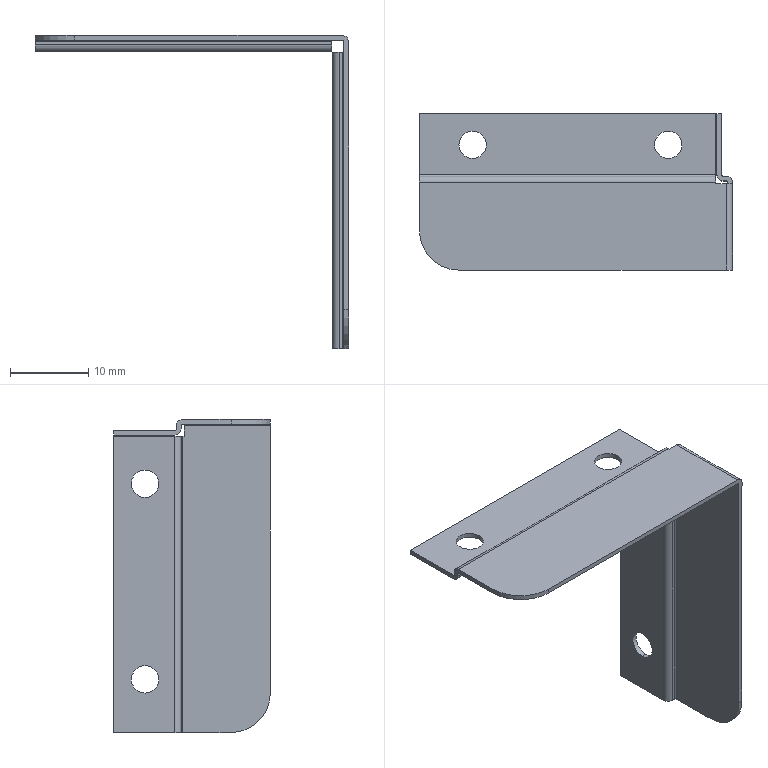Part | SolidWorks | features BaseBody 1 | 1 solid | 40 faces | box 40 x 20 x 40 mm | volume 945.968 mm3 | cylinder 20 | plane 20 | commonest cylinder face diameters 3.5 x8 0.4 x5 1.6 x5 10 x2
STEP:
#1=CARTESIAN_POINT('',(-9.96,6.,-2.));
#2=VERTEX_POINT('',#1);
#3=CARTESIAN_POINT('',(-6.46,6.,-2.));
#4=VERTEX_POINT('',#3);
#5=CARTESIAN_POINT('',(-8.21,6.,-2.));
#6=DIRECTION('',(0.,0.,1.));
#7=DIRECTION('',(1.,0.,0.));
#8=AXIS2_PLACEMENT_3D('',#5,#6,#7);
#9=CIRCLE('',#8,1.75);
#10=EDGE_CURVE('',#2,#4,#9,.T.);
#11=ORIENTED_EDGE('',*,*,#10,.F.);
#12=CARTESIAN_POINT('',(-9.96,6.,-1.4));
#13=VERTEX_POINT('',#12);
#14=CARTESIAN_POINT('',(-9.96,6.,-2.));
#15=DIRECTION('',(0.,0.,1.));
#16=VECTOR('',#15,1000.);
#17=LINE('',#14,#16);
#18=EDGE_CURVE('',#2,#13,#17,.T.);
#19=ORIENTED_EDGE('',*,*,#18,.T.);
#20=CARTESIAN_POINT('',(-6.46,6.,-1.4));
#21=VERTEX_POINT('',#20);
#22=CARTESIAN_POINT('',(-8.21,6.,-1.4));
#23=DIRECTION('',(0.,0.,-1.));
#24=DIRECTION('',(1.,0.,0.));
#25=AXIS2_PLACEMENT_3D('',#22,#23,#24);
#26=CIRCLE('',#25,1.75);
#27=EDGE_CURVE('',#21,#13,#26,.T.);
#28=ORIENTED_EDGE('',*,*,#27,.F.);
#29=CARTESIAN_POINT('',(-6.46,6.,-2.));
#30=DIRECTION('',(0.,0.,1.));
#31=VECTOR('',#30,1000.);
#32=LINE('',#29,#31);
#33=EDGE_CURVE('',#4,#21,#32,.T.);
#34=ORIENTED_EDGE('',*,*,#33,.F.);
#35=EDGE_LOOP('',(#11,#19,#28,#34));
#36=FACE_OUTER_BOUND('',#35,.T.);
#37=CARTESIAN_POINT('',(-8.21,6.,-2.));
#38=DIRECTION('',(0.,0.,1.));
#39=DIRECTION('',(1.,0.,0.));
#40=AXIS2_PLACEMENT_3D('',#37,#38,#39);
#41=CYLINDRICAL_SURFACE('',#40,1.75);
#42=ADVANCED_FACE('',(#36),#41,.F.);
#43=CARTESIAN_POINT('',(-34.96,6.,-2.));
#44=VERTEX_POINT('',#43);
#45=CARTESIAN_POINT('',(-31.46,6.,-2.));
#46=VERTEX_POINT('',#45);
#47=CARTESIAN_POINT('',(-33.21,6.,-2.));
#48=DIRECTION('',(0.,0.,1.));
#49=DIRECTION('',(1.,0.,0.));
#50=AXIS2_PLACEMENT_3D('',#47,#48,#49);
#51=CIRCLE('',#50,1.75);
#52=EDGE_CURVE('',#44,#46,#51,.T.);
#53=ORIENTED_EDGE('',*,*,#52,.F.);
#54=CARTESIAN_POINT('',(-34.96,6.,-1.4));
#55=VERTEX_POINT('',#54);
#56=CARTESIAN_POINT('',(-34.96,6.,-2.));
#57=DIRECTION('',(0.,0.,1.));
#58=VECTOR('',#57,1000.);
#59=LINE('',#56,#58);
#60=EDGE_CURVE('',#44,#55,#59,.T.);
#61=ORIENTED_EDGE('',*,*,#60,.T.);
#62=CARTESIAN_POINT('',(-31.46,6.,-1.4));
#63=VERTEX_POINT('',#62);
#64=CARTESIAN_POINT('',(-33.21,6.,-1.4));
#65=DIRECTION('',(0.,0.,-1.));
#66=DIRECTION('',(1.,0.,0.));
#67=AXIS2_PLACEMENT_3D('',#64,#65,#66);
#68=CIRCLE('',#67,1.75);
#69=EDGE_CURVE('',#63,#55,#68,.T.);
#70=ORIENTED_EDGE('',*,*,#69,.F.);
#71=CARTESIAN_POINT('',(-31.46,6.,-2.));
#72=DIRECTION('',(0.,0.,1.));
#73=VECTOR('',#72,1000.);
#74=LINE('',#71,#73);
#75=EDGE_CURVE('',#46,#63,#74,.T.);
#76=ORIENTED_EDGE('',*,*,#75,.F.);
#77=EDGE_LOOP('',(#53,#61,#70,#76));
#78=FACE_OUTER_BOUND('',#77,.T.);
#79=CARTESIAN_POINT('',(-33.21,6.,-2.));
#80=DIRECTION('',(0.,0.,1.));
#81=DIRECTION('',(1.,0.,0.));
#82=AXIS2_PLACEMENT_3D('',#79,#80,#81);
#83=CYLINDRICAL_SURFACE('',#82,1.75);
#84=ADVANCED_FACE('',(#78),#83,.F.);
#85=CARTESIAN_POINT('',(-2.,6.,-6.46));
#86=VERTEX_POINT('',#85);
#87=CARTESIAN_POINT('',(-2.,6.,-9.96));
#88=VERTEX_POINT('',#87);
#89=CARTESIAN_POINT('',(-2.,6.,-8.21));
#90=DIRECTION('',(1.,0.,0.));
#91=DIRECTION('',(0.,0.,-1.));
#92=AXIS2_PLACEMENT_3D('',#89,#90,#91);
#93=CIRCLE('',#92,1.75);
#94=EDGE_CURVE('',#86,#88,#93,.T.);
#95=ORIENTED_EDGE('',*,*,#94,.F.);
#96=CARTESIAN_POINT('',(-1.4,6.,-6.46));
#97=VERTEX_POINT('',#96);
#98=CARTESIAN_POINT('',(-2.,6.,-6.46));
#99=DIRECTION('',(1.,0.,0.));
#100=VECTOR('',#99,1000.);
#101=LINE('',#98,#100);
#102=EDGE_CURVE('',#86,#97,#101,.T.);
#103=ORIENTED_EDGE('',*,*,#102,.T.);
#104=CARTESIAN_POINT('',(-1.4,6.,-9.96));
#105=VERTEX_POINT('',#104);
#106=CARTESIAN_POINT('',(-1.4,6.,-8.21));
#107=DIRECTION('',(-1.,0.,0.));
#108=DIRECTION('',(0.,0.,-1.));
#109=AXIS2_PLACEMENT_3D('',#106,#107,#108);
#110=CIRCLE('',#109,1.75);
#111=EDGE_CURVE('',#105,#97,#110,.T.);
#112=ORIENTED_EDGE('',*,*,#111,.F.);
#113=CARTESIAN_POINT('',(-2.,6.,-9.96));
#114=DIRECTION('',(1.,0.,0.));
#115=VECTOR('',#114,1000.);
#116=LINE('',#113,#115);
#117=EDGE_CURVE('',#88,#105,#116,.T.);
#118=ORIENTED_EDGE('',*,*,#117,.F.);
#119=EDGE_LOOP('',(#95,#103,#112,#118));
#120=FACE_OUTER_BOUND('',#119,.T.);
#121=CARTESIAN_POINT('',(-2.,6.,-8.21));
#122=DIRECTION('',(1.,0.,0.));
#123=DIRECTION('',(0.,0.,-1.));
#124=AXIS2_PLACEMENT_3D('',#121,#122,#123);
#125=CYLINDRICAL_SURFACE('',#124,1.75);
#126=ADVANCED_FACE('',(#120),#125,.F.);
#127=CARTESIAN_POINT('',(-2.,6.,-31.46));
#128=VERTEX_POINT('',#127);
#129=CARTESIAN_POINT('',(-2.,6.,-34.96));
#130=VERTEX_POINT('',#129);
#131=CARTESIAN_POINT('',(-2.,6.,-33.21));
#132=DIRECTION('',(1.,0.,0.));
#133=DIRECTION('',(0.,0.,-1.));
#134=AXIS2_PLACEMENT_3D('',#131,#132,#133);
#135=CIRCLE('',#134,1.75);
#136=EDGE_CURVE('',#128,#130,#135,.T.);
#137=ORIENTED_EDGE('',*,*,#136,.F.);
#138=CARTESIAN_POINT('',(-1.4,6.,-31.46));
#139=VERTEX_POINT('',#138);
#140=CARTESIAN_POINT('',(-2.,6.,-31.46));
#141=DIRECTION('',(1.,0.,0.));
#142=VECTOR('',#141,1000.);
#143=LINE('',#140,#142);
#144=EDGE_CURVE('',#128,#139,#143,.T.);
#145=ORIENTED_EDGE('',*,*,#144,.T.);
#146=CARTESIAN_POINT('',(-1.4,6.,-34.96));
#147=VERTEX_POINT('',#146);
#148=CARTESIAN_POINT('',(-1.4,6.,-33.21));
#149=DIRECTION('',(-1.,0.,0.));
#150=DIRECTION('',(0.,0.,-1.));
#151=AXIS2_PLACEMENT_3D('',#148,#149,#150);
#152=CIRCLE('',#151,1.75);
#153=EDGE_CURVE('',#147,#139,#152,.T.);
#154=ORIENTED_EDGE('',*,*,#153,.F.);
#155=CARTESIAN_POINT('',(-2.,6.,-34.96));
#156=DIRECTION('',(1.,0.,0.));
#157=VECTOR('',#156,1000.);
#158=LINE('',#155,#157);
#159=EDGE_CURVE('',#130,#147,#158,.T.);
#160=ORIENTED_EDGE('',*,*,#159,.F.);
#161=EDGE_LOOP('',(#137,#145,#154,#160));
#162=FACE_OUTER_BOUND('',#161,.T.);
#163=CARTESIAN_POINT('',(-2.,6.,-33.21));
#164=DIRECTION('',(1.,0.,0.));
#165=DIRECTION('',(0.,0.,-1.));
#166=AXIS2_PLACEMENT_3D('',#163,#164,#165);
#167=CYLINDRICAL_SURFACE('',#166,1.75);
#168=ADVANCED_FACE('',(#162),#167,.F.);
#169=CARTESIAN_POINT('',(-0.8,-10.,0.));
#170=VERTEX_POINT('',#169);
#171=CARTESIAN_POINT('',(-0.8,1.,0.));
#172=VERTEX_POINT('',#171);
#173=CARTESIAN_POINT('',(-0.8,10.,0.));
#174=DIRECTION('',(0.,1.,0.));
#175=VECTOR('',#174,1000.);
#176=LINE('',#173,#175);
#177=EDGE_CURVE('',#170,#172,#176,.T.);
#178=ORIENTED_EDGE('',*,*,#177,.T.);
#179=CARTESIAN_POINT('',(-2.15,1.,0.));
#180=VERTEX_POINT('',#179);
#181=CARTESIAN_POINT('',(0.,1.,0.));
#182=DIRECTION('',(-1.,0.,0.));
#183=VECTOR('',#182,1000.);
#184=LINE('',#181,#183);
#185=EDGE_CURVE('',#172,#180,#184,.T.);
#186=ORIENTED_EDGE('',*,*,#185,.T.);
#187=CARTESIAN_POINT('',(-2.15,1.2,0.));
#188=VERTEX_POINT('',#187);
#189=CARTESIAN_POINT('',(-2.15,10.,0.));
#190=DIRECTION('',(0.,1.,0.));
#191=VECTOR('',#190,1000.);
#192=LINE('',#189,#191);
#193=EDGE_CURVE('',#180,#188,#192,.T.);
#194=ORIENTED_EDGE('',*,*,#193,.T.);
#195=CARTESIAN_POINT('',(-40.,1.2,0.));
#196=VERTEX_POINT('',#195);
#197=CARTESIAN_POINT('',(0.,1.2,0.));
#198=DIRECTION('',(-1.,0.,0.));
#199=VECTOR('',#198,1000.);
#200=LINE('',#197,#199);
#201=EDGE_CURVE('',#188,#196,#200,.T.);
#202=ORIENTED_EDGE('',*,*,#201,.T.);
#203=CARTESIAN_POINT('',(-40.,-5.,0.));
#204=VERTEX_POINT('',#203);
#205=CARTESIAN_POINT('',(-40.,10.,0.));
#206=DIRECTION('',(0.,-1.,0.));
#207=VECTOR('',#206,1000.);
#208=LINE('',#205,#207);
#209=EDGE_CURVE('',#196,#204,#208,.T.);
#210=ORIENTED_EDGE('',*,*,#209,.T.);
#211=CARTESIAN_POINT('',(-35.,-10.,0.));
#212=VERTEX_POINT('',#211);
#213=CARTESIAN_POINT('',(-35.,-5.,0.));
#214=DIRECTION('',(0.,0.,1.));
#215=DIRECTION('',(1.,0.,0.));
#216=AXIS2_PLACEMENT_3D('',#213,#214,#215);
#217=CIRCLE('',#216,5.);
#218=EDGE_CURVE('',#204,#212,#217,.T.);
#219=ORIENTED_EDGE('',*,*,#218,.T.);
#220=CARTESIAN_POINT('',(0.,-10.,0.));
#221=DIRECTION('',(1.,0.,0.));
#222=VECTOR('',#221,1000.);
#223=LINE('',#220,#222);
#224=EDGE_CURVE('',#212,#170,#223,.T.);
#225=ORIENTED_EDGE('',*,*,#224,.T.);
#226=EDGE_LOOP('',(#178,#186,#194,#202,#210,#219,#225));
#227=FACE_OUTER_BOUND('',#226,.T.);
#228=CARTESIAN_POINT('',(0.,10.,0.));
#229=DIRECTION('',(0.,0.,1.));
#230=DIRECTION('',(1.,0.,0.));
#231=AXIS2_PLACEMENT_3D('',#228,#229,#230);
#232=PLANE('',#231);
#233=ADVANCED_FACE('',(#227),#232,.T.);
#234=CARTESIAN_POINT('',(-0.8,1.,-0.6));
#235=VERTEX_POINT('',#234);
#236=CARTESIAN_POINT('',(-2.15,1.,-0.6));
#237=VERTEX_POINT('',#236);
#238=CARTESIAN_POINT('',(0.,1.,-0.6));
#239=DIRECTION('',(-1.,0.,0.));
#240=VECTOR('',#239,1000.);
#241=LINE('',#238,#240);
#242=EDGE_CURVE('',#235,#237,#241,.T.);
#243=ORIENTED_EDGE('',*,*,#242,.T.);
#244=CARTESIAN_POINT('',(-2.15,1.,0.));
#245=DIRECTION('',(0.,0.,1.));
#246=VECTOR('',#245,1000.);
#247=LINE('',#244,#246);
#248=EDGE_CURVE('',#237,#180,#247,.T.);
#249=ORIENTED_EDGE('',*,*,#248,.T.);
#250=ORIENTED_EDGE('',*,*,#185,.F.);
#251=CARTESIAN_POINT('',(0.,1.,-0.8));
#252=VERTEX_POINT('',#251);
#253=CARTESIAN_POINT('',(-0.8,1.,-0.8));
#254=DIRECTION('',(0.,-1.,0.));
#255=DIRECTION('',(0.,0.,-1.));
#256=AXIS2_PLACEMENT_3D('',#253,#254,#255);
#257=CIRCLE('',#256,0.8);
#258=EDGE_CURVE('',#252,#172,#257,.T.);
#259=ORIENTED_EDGE('',*,*,#258,.F.);
#260=CARTESIAN_POINT('',(0.,1.,-2.15));
#261=VERTEX_POINT('',#260);
#262=CARTESIAN_POINT('',(0.,1.,0.));
#263=DIRECTION('',(0.,0.,1.));
#264=VECTOR('',#263,1000.);
#265=LINE('',#262,#264);
#266=EDGE_CURVE('',#261,#252,#265,.T.);
#267=ORIENTED_EDGE('',*,*,#266,.F.);
#268=CARTESIAN_POINT('',(-0.6,1.,-2.15));
#269=VERTEX_POINT('',#268);
#270=CARTESIAN_POINT('',(0.,1.,-2.15));
#271=DIRECTION('',(-1.,0.,0.));
#272=VECTOR('',#271,1000.);
#273=LINE('',#270,#272);
#274=EDGE_CURVE('',#261,#269,#273,.T.);
#275=ORIENTED_EDGE('',*,*,#274,.T.);
#276=CARTESIAN_POINT('',(-0.6,1.,-0.8));
#277=VERTEX_POINT('',#276);
#278=CARTESIAN_POINT('',(-0.6,1.,0.));
#279=DIRECTION('',(0.,0.,1.));
#280=VECTOR('',#279,1000.);
#281=LINE('',#278,#280);
#282=EDGE_CURVE('',#269,#277,#281,.T.);
#283=ORIENTED_EDGE('',*,*,#282,.T.);
#284=CARTESIAN_POINT('',(-0.8,1.,-0.8));
#285=DIRECTION('',(0.,-1.,0.));
#286=DIRECTION('',(0.,0.,-1.));
#287=AXIS2_PLACEMENT_3D('',#284,#285,#286);
#288=CIRCLE('',#287,0.2);
#289=EDGE_CURVE('',#277,#235,#288,.T.);
#290=ORIENTED_EDGE('',*,*,#289,.T.);
#291=EDGE_LOOP('',(#243,#249,#250,#259,#267,#275,#283,#290));
#292=FACE_OUTER_BOUND('',#291,.T.);
#293=CARTESIAN_POINT('',(0.,1.,0.));
#294=DIRECTION('',(0.,1.,0.));
#295=DIRECTION('',(0.,0.,1.));
#296=AXIS2_PLACEMENT_3D('',#293,#294,#295);
#297=PLANE('',#296);
#298=ADVANCED_FACE('',(#292),#297,.T.);
#299=ORIENTED_EDGE('',*,*,#177,.F.);
#300=CARTESIAN_POINT('',(0.,-10.,-0.8));
#301=VERTEX_POINT('',#300);
#302=CARTESIAN_POINT('',(-0.8,-10.,-0.8));
#303=DIRECTION('',(0.,1.,0.));
#304=DIRECTION('',(0.,0.,-1.));
#305=AXIS2_PLACEMENT_3D('',#302,#303,#304);
#306=CIRCLE('',#305,0.8);
#307=EDGE_CURVE('',#170,#301,#306,.T.);
#308=ORIENTED_EDGE('',*,*,#307,.T.);
#309=CARTESIAN_POINT('',(0.,10.,-0.8));
#310=DIRECTION('',(0.,1.,0.));
#311=VECTOR('',#310,1000.);
#312=LINE('',#309,#311);
#313=EDGE_CURVE('',#301,#252,#312,.T.);
#314=ORIENTED_EDGE('',*,*,#313,.T.);
#315=ORIENTED_EDGE('',*,*,#258,.T.);
#316=EDGE_LOOP('',(#299,#308,#314,#315));
#317=FACE_OUTER_BOUND('',#316,.T.);
#318=CARTESIAN_POINT('',(-0.8,10.,-0.8));
#319=DIRECTION('',(0.,-1.,0.));
#320=DIRECTION('',(0.,0.,-1.));
#321=AXIS2_PLACEMENT_3D('',#318,#319,#320);
#322=CYLINDRICAL_SURFACE('',#321,0.8);
#323=ADVANCED_FACE('',(#317),#322,.T.);
#324=CARTESIAN_POINT('',(-35.,-10.,-0.6));
#325=VERTEX_POINT('',#324);
#326=CARTESIAN_POINT('',(-35.,-10.,-0.8));
#327=DIRECTION('',(0.,0.,1.));
#328=VECTOR('',#327,1000.);
#329=LINE('',#326,#328);
#330=EDGE_CURVE('',#325,#212,#329,.T.);
#331=ORIENTED_EDGE('',*,*,#330,.F.);
#332=CARTESIAN_POINT('',(-0.8,-10.,-0.6));
#333=VERTEX_POINT('',#332);
#334=CARTESIAN_POINT('',(-0.8,-10.,-0.6));
#335=DIRECTION('',(-1.,0.,0.));
#336=VECTOR('',#335,1000.);
#337=LINE('',#334,#336);
#338=EDGE_CURVE('',#333,#325,#337,.T.);
#339=ORIENTED_EDGE('',*,*,#338,.F.);
#340=CARTESIAN_POINT('',(-0.6,-10.,-0.8));
#341=VERTEX_POINT('',#340);
#342=CARTESIAN_POINT('',(-0.8,-10.,-0.8));
#343=DIRECTION('',(0.,1.,0.));
#344=DIRECTION('',(0.,0.,-1.));
#345=AXIS2_PLACEMENT_3D('',#342,#343,#344);
#346=CIRCLE('',#345,0.2);
#347=EDGE_CURVE('',#333,#341,#346,.T.);
#348=ORIENTED_EDGE('',*,*,#347,.T.);
#349=CARTESIAN_POINT('',(-0.6,-10.,-35.));
#350=VERTEX_POINT('',#349);
#351=CARTESIAN_POINT('',(-0.6,-10.,-0.6));
#352=DIRECTION('',(0.,0.,-1.));
#353=VECTOR('',#352,1000.);
#354=LINE('',#351,#353);
#355=EDGE_CURVE('',#341,#350,#354,.T.);
#356=ORIENTED_EDGE('',*,*,#355,.T.);
#357=CARTESIAN_POINT('',(0.,-10.,-35.));
#358=VERTEX_POINT('',#357);
#359=CARTESIAN_POINT('',(-0.8,-10.,-35.));
#360=DIRECTION('',(-1.,0.,0.));
#361=VECTOR('',#360,1000.);
#362=LINE('',#359,#361);
#363=EDGE_CURVE('',#358,#350,#362,.T.);
#364=ORIENTED_EDGE('',*,*,#363,.F.);
#365=CARTESIAN_POINT('',(0.,-10.,0.));
#366=DIRECTION('',(0.,0.,-1.));
#367=VECTOR('',#366,1000.);
#368=LINE('',#365,#367);
#369=EDGE_CURVE('',#301,#358,#368,.T.);
#370=ORIENTED_EDGE('',*,*,#369,.F.);
#371=ORIENTED_EDGE('',*,*,#307,.F.);
#372=ORIENTED_EDGE('',*,*,#224,.F.);
#373=EDGE_LOOP('',(#331,#339,#348,#356,#364,#370,#371,#372));
#374=FACE_OUTER_BOUND('',#373,.T.);
#375=CARTESIAN_POINT('',(-0.8,-10.,-0.8));
#376=DIRECTION('',(0.,1.,0.));
#377=DIRECTION('',(0.,0.,1.));
#378=AXIS2_PLACEMENT_3D('',#375,#376,#377);
#379=PLANE('',#378);
#380=ADVANCED_FACE('',(#374),#379,.F.);
#381=CARTESIAN_POINT('',(-40.,-5.,-0.6));
#382=VERTEX_POINT('',#381);
#383=CARTESIAN_POINT('',(-35.,-5.,-0.6));
#384=DIRECTION('',(0.,0.,1.));
#385=DIRECTION('',(1.,0.,0.));
#386=AXIS2_PLACEMENT_3D('',#383,#384,#385);
#387=CIRCLE('',#386,5.);
#388=EDGE_CURVE('',#382,#325,#387,.T.);
#389=ORIENTED_EDGE('',*,*,#388,.T.);
#390=ORIENTED_EDGE('',*,*,#330,.T.);
#391=ORIENTED_EDGE('',*,*,#218,.F.);
#392=CARTESIAN_POINT('',(-40.,-5.,-0.8));
#393=DIRECTION('',(0.,0.,-1.));
#394=VECTOR('',#393,1000.);
#395=LINE('',#392,#394);
#396=EDGE_CURVE('',#204,#382,#395,.T.);
#397=ORIENTED_EDGE('',*,*,#396,.T.);
#398=EDGE_LOOP('',(#389,#390,#391,#397));
#399=FACE_OUTER_BOUND('',#398,.T.);
#400=CARTESIAN_POINT('',(-35.,-5.,-0.8));
#401=DIRECTION('',(0.,0.,1.));
#402=DIRECTION('',(1.,0.,0.));
#403=AXIS2_PLACEMENT_3D('',#400,#401,#402);
#404=CYLINDRICAL_SURFACE('',#403,5.);
#405=ADVANCED_FACE('',(#399),#404,.T.);
#406=CARTESIAN_POINT('',(-40.,1.2,-0.6));
#407=VERTEX_POINT('',#406);
#408=CARTESIAN_POINT('',(-40.,10.,-0.6));
#409=DIRECTION('',(0.,-1.,0.));
#410=VECTOR('',#409,1000.);
#411=LINE('',#408,#410);
#412=EDGE_CURVE('',#407,#382,#411,.T.);
#413=ORIENTED_EDGE('',*,*,#412,.T.);
#414=ORIENTED_EDGE('',*,*,#396,.F.);
#415=ORIENTED_EDGE('',*,*,#209,.F.);
#416=CARTESIAN_POINT('',(-40.,2.,-0.8));
#417=VERTEX_POINT('',#416);
#418=CARTESIAN_POINT('',(-40.,1.2,-0.8));
#419=DIRECTION('',(1.,0.,0.));
#420=DIRECTION('',(0.,0.,1.));
#421=AXIS2_PLACEMENT_3D('',#418,#419,#420);
#422=CIRCLE('',#421,0.8);
#423=EDGE_CURVE('',#417,#196,#422,.T.);
#424=ORIENTED_EDGE('',*,*,#423,.F.);
#425=CARTESIAN_POINT('',(-40.,2.,-1.2));
#426=VERTEX_POINT('',#425);
#427=CARTESIAN_POINT('',(-40.,2.,-8.923));
#428=DIRECTION('',(0.,0.,1.));
#429=VECTOR('',#428,1000.);
#430=LINE('',#427,#429);
#431=EDGE_CURVE('',#426,#417,#430,.T.);
#432=ORIENTED_EDGE('',*,*,#431,.F.);
#433=CARTESIAN_POINT('',(-40.,2.2,-1.4));
#434=VERTEX_POINT('',#433);
#435=CARTESIAN_POINT('',(-40.,2.2,-1.2));
#436=DIRECTION('',(1.,0.,0.));
#437=DIRECTION('',(0.,0.,1.));
#438=AXIS2_PLACEMENT_3D('',#435,#436,#437);
#439=CIRCLE('',#438,0.2);
#440=EDGE_CURVE('',#426,#434,#439,.T.);
#441=ORIENTED_EDGE('',*,*,#440,.T.);
#442=CARTESIAN_POINT('',(-40.,10.,-1.4));
#443=VERTEX_POINT('',#442);
#444=CARTESIAN_POINT('',(-40.,9.246,-1.4));
#445=DIRECTION('',(0.,-1.,0.));
#446=VECTOR('',#445,1000.);
#447=LINE('',#444,#446);
#448=EDGE_CURVE('',#443,#434,#447,.T.);
#449=ORIENTED_EDGE('',*,*,#448,.F.);
#450=CARTESIAN_POINT('',(-40.,10.,-2.));
#451=VERTEX_POINT('',#450);
#452=CARTESIAN_POINT('',(-40.,10.,-1.4));
#453=DIRECTION('',(0.,0.,-1.));
#454=VECTOR('',#453,1000.);
#455=LINE('',#452,#454);
#456=EDGE_CURVE('',#443,#451,#455,.T.);
#457=ORIENTED_EDGE('',*,*,#456,.T.);
#458=CARTESIAN_POINT('',(-40.,2.2,-2.));
#459=VERTEX_POINT('',#458);
#460=CARTESIAN_POINT('',(-40.,9.246,-2.));
#461=DIRECTION('',(0.,-1.,0.));
#462=VECTOR('',#461,1000.);
#463=LINE('',#460,#462);
#464=EDGE_CURVE('',#451,#459,#463,.T.);
#465=ORIENTED_EDGE('',*,*,#464,.T.);
#466=CARTESIAN_POINT('',(-40.,1.4,-1.2));
#467=VERTEX_POINT('',#466);
#468=CARTESIAN_POINT('',(-40.,2.2,-1.2));
#469=DIRECTION('',(1.,0.,0.));
#470=DIRECTION('',(0.,0.,1.));
#471=AXIS2_PLACEMENT_3D('',#468,#469,#470);
#472=CIRCLE('',#471,0.8);
#473=EDGE_CURVE('',#467,#459,#472,.T.);
#474=ORIENTED_EDGE('',*,*,#473,.F.);
#475=CARTESIAN_POINT('',(-40.,1.4,-0.8));
#476=VERTEX_POINT('',#475);
#477=CARTESIAN_POINT('',(-40.,1.4,-8.923));
#478=DIRECTION('',(0.,0.,1.));
#479=VECTOR('',#478,1000.);
#480=LINE('',#477,#479);
#481=EDGE_CURVE('',#467,#476,#480,.T.);
#482=ORIENTED_EDGE('',*,*,#481,.T.);
#483=CARTESIAN_POINT('',(-40.,1.2,-0.8));
#484=DIRECTION('',(1.,0.,0.));
#485=DIRECTION('',(0.,0.,1.));
#486=AXIS2_PLACEMENT_3D('',#483,#484,#485);
#487=CIRCLE('',#486,0.2);
#488=EDGE_CURVE('',#476,#407,#487,.T.);
#489=ORIENTED_EDGE('',*,*,#488,.T.);
#490=EDGE_LOOP('',(#413,#414,#415,#424,#432,#441,#449,#457,#465,#474,#482,#489));
#491=FACE_OUTER_BOUND('',#490,.T.);
#492=CARTESIAN_POINT('',(-40.,10.,0.));
#493=DIRECTION('',(-1.,0.,0.));
#494=DIRECTION('',(0.,0.,1.));
#495=AXIS2_PLACEMENT_3D('',#492,#493,#494);
#496=PLANE('',#495);
#497=ADVANCED_FACE('',(#491),#496,.T.);
#498=CARTESIAN_POINT('',(-2.15,2.,-0.8));
#499=VERTEX_POINT('',#498);
#500=CARTESIAN_POINT('',(-2.15,1.2,-0.8));
#501=DIRECTION('',(-1.,0.,0.));
#502=DIRECTION('',(0.,0.,1.));
#503=AXIS2_PLACEMENT_3D('',#500,#501,#502);
#504=CIRCLE('',#503,0.8);
#505=EDGE_CURVE('',#188,#499,#504,.T.);
#506=ORIENTED_EDGE('',*,*,#505,.T.);
#507=CARTESIAN_POINT('',(16.786,2.,-0.8));
#508=DIRECTION('',(-1.,0.,0.));
#509=VECTOR('',#508,1000.);
#510=LINE('',#507,#509);
#511=EDGE_CURVE('',#499,#417,#510,.T.);
#512=ORIENTED_EDGE('',*,*,#511,.T.);
#513=ORIENTED_EDGE('',*,*,#423,.T.);
#514=ORIENTED_EDGE('',*,*,#201,.F.);
#515=EDGE_LOOP('',(#506,#512,#513,#514));
#516=FACE_OUTER_BOUND('',#515,.T.);
#517=CARTESIAN_POINT('',(16.786,1.2,-0.8));
#518=DIRECTION('',(-1.,0.,0.));
#519=DIRECTION('',(0.,0.,1.));
#520=AXIS2_PLACEMENT_3D('',#517,#518,#519);
#521=CYLINDRICAL_SURFACE('',#520,0.8);
#522=ADVANCED_FACE('',(#516),#521,.T.);
#523=ORIENTED_EDGE('',*,*,#193,.F.);
#524=ORIENTED_EDGE('',*,*,#248,.F.);
#525=CARTESIAN_POINT('',(-2.15,1.2,-0.6));
#526=VERTEX_POINT('',#525);
#527=CARTESIAN_POINT('',(-2.15,1.,-0.6));
#528=DIRECTION('',(0.,-1.,0.));
#529=VECTOR('',#528,1000.);
#530=LINE('',#527,#529);
#531=EDGE_CURVE('',#526,#237,#530,.T.);
#532=ORIENTED_EDGE('',*,*,#531,.F.);
#533=CARTESIAN_POINT('',(-2.15,1.4,-0.8));
#534=VERTEX_POINT('',#533);
#535=CARTESIAN_POINT('',(-2.15,1.2,-0.8));
#536=DIRECTION('',(-1.,0.,0.));
#537=DIRECTION('',(0.,0.,1.));
#538=AXIS2_PLACEMENT_3D('',#535,#536,#537);
#539=CIRCLE('',#538,0.2);
#540=EDGE_CURVE('',#526,#534,#539,.T.);
#541=ORIENTED_EDGE('',*,*,#540,.T.);
#542=CARTESIAN_POINT('',(-2.15,1.4,-1.2));
#543=VERTEX_POINT('',#542);
#544=CARTESIAN_POINT('',(-2.15,1.4,0.07701));
#545=DIRECTION('',(0.,0.,1.));
#546=VECTOR('',#545,1000.);
#547=LINE('',#544,#546);
#548=EDGE_CURVE('',#543,#534,#547,.T.);
#549=ORIENTED_EDGE('',*,*,#548,.F.);
#550=CARTESIAN_POINT('',(-2.15,2.2,-2.));
#551=VERTEX_POINT('',#550);
#552=CARTESIAN_POINT('',(-2.15,2.2,-1.2));
#553=DIRECTION('',(-1.,0.,0.));
#554=DIRECTION('',(0.,0.,1.));
#555=AXIS2_PLACEMENT_3D('',#552,#553,#554);
#556=CIRCLE('',#555,0.8);
#557=EDGE_CURVE('',#551,#543,#556,.T.);
#558=ORIENTED_EDGE('',*,*,#557,.F.);
#559=CARTESIAN_POINT('',(-2.15,10.,-2.));
#560=VERTEX_POINT('',#559);
#561=CARTESIAN_POINT('',(-2.15,0.246,-2.));
#562=DIRECTION('',(0.,-1.,0.));
#563=VECTOR('',#562,1000.);
#564=LINE('',#561,#563);
#565=EDGE_CURVE('',#560,#551,#564,.T.);
#566=ORIENTED_EDGE('',*,*,#565,.F.);
#567=CARTESIAN_POINT('',(-2.15,10.,-1.4));
#568=VERTEX_POINT('',#567);
#569=CARTESIAN_POINT('',(-2.15,10.,-2.2));
#570=DIRECTION('',(0.,0.,-1.));
#571=VECTOR('',#570,1000.);
#572=LINE('',#569,#571);
#573=EDGE_CURVE('',#568,#560,#572,.T.);
#574=ORIENTED_EDGE('',*,*,#573,.F.);
#575=CARTESIAN_POINT('',(-2.15,2.2,-1.4));
#576=VERTEX_POINT('',#575);
#577=CARTESIAN_POINT('',(-2.15,9.246,-1.4));
#578=DIRECTION('',(0.,1.,0.));
#579=VECTOR('',#578,1000.);
#580=LINE('',#577,#579);
#581=EDGE_CURVE('',#576,#568,#580,.T.);
#582=ORIENTED_EDGE('',*,*,#581,.F.);
#583=CARTESIAN_POINT('',(-2.15,2.,-1.2));
#584=VERTEX_POINT('',#583);
#585=CARTESIAN_POINT('',(-2.15,2.2,-1.2));
#586=DIRECTION('',(-1.,0.,0.));
#587=DIRECTION('',(0.,0.,1.));
#588=AXIS2_PLACEMENT_3D('',#585,#586,#587);
#589=CIRCLE('',#588,0.2);
#590=EDGE_CURVE('',#576,#584,#589,.T.);
#591=ORIENTED_EDGE('',*,*,#590,.T.);
#592=CARTESIAN_POINT('',(-2.15,2.,-8.923));
#593=DIRECTION('',(0.,0.,-1.));
#594=VECTOR('',#593,1000.);
#595=LINE('',#592,#594);
#596=EDGE_CURVE('',#499,#584,#595,.T.);
#597=ORIENTED_EDGE('',*,*,#596,.F.);
#598=ORIENTED_EDGE('',*,*,#505,.F.);
#599=EDGE_LOOP('',(#523,#524,#532,#541,#549,#558,#566,#574,#582,#591,#597,#598));
#600=FACE_OUTER_BOUND('',#599,.T.);
#601=CARTESIAN_POINT('',(-2.15,1.,-2.15));
#602=DIRECTION('',(-1.,0.,0.));
#603=DIRECTION('',(0.,0.,1.));
#604=AXIS2_PLACEMENT_3D('',#601,#602,#603);
#605=PLANE('',#604);
#606=ADVANCED_FACE('',(#600),#605,.F.);
#607=ORIENTED_EDGE('',*,*,#369,.T.);
#608=CARTESIAN_POINT('',(0.,-5.,-40.));
#609=VERTEX_POINT('',#608);
#610=CARTESIAN_POINT('',(0.,-5.,-35.));
#611=DIRECTION('',(1.,0.,0.));
#612=DIRECTION('',(0.,0.,-1.));
#613=AXIS2_PLACEMENT_3D('',#610,#611,#612);
#614=CIRCLE('',#613,5.);
#615=EDGE_CURVE('',#358,#609,#614,.T.);
#616=ORIENTED_EDGE('',*,*,#615,.T.);
#617=CARTESIAN_POINT('',(0.,1.2,-40.));
#618=VERTEX_POINT('',#617);
#619=CARTESIAN_POINT('',(0.,10.,-40.));
#620=DIRECTION('',(0.,1.,0.));
#621=VECTOR('',#620,1000.);
#622=LINE('',#619,#621);
#623=EDGE_CURVE('',#609,#618,#622,.T.);
#624=ORIENTED_EDGE('',*,*,#623,.T.);
#625=CARTESIAN_POINT('',(0.,1.2,-2.15));
#626=VERTEX_POINT('',#625);
#627=CARTESIAN_POINT('',(0.,1.2,0.));
#628=DIRECTION('',(0.,0.,1.));
#629=VECTOR('',#628,1000.);
#630=LINE('',#627,#629);
#631=EDGE_CURVE('',#618,#626,#630,.T.);
#632=ORIENTED_EDGE('',*,*,#631,.T.);
#633=CARTESIAN_POINT('',(0.,10.,-2.15));
#634=DIRECTION('',(0.,-1.,0.));
#635=VECTOR('',#634,1000.);
#636=LINE('',#633,#635);
#637=EDGE_CURVE('',#626,#261,#636,.T.);
#638=ORIENTED_EDGE('',*,*,#637,.T.);
#639=ORIENTED_EDGE('',*,*,#266,.T.);
#640=ORIENTED_EDGE('',*,*,#313,.F.);
#641=EDGE_LOOP('',(#607,#616,#624,#632,#638,#639,#640));
#642=FACE_OUTER_BOUND('',#641,.T.);
#643=CARTESIAN_POINT('',(0.,10.,0.));
#644=DIRECTION('',(1.,0.,0.));
#645=DIRECTION('',(0.,0.,-1.));
#646=AXIS2_PLACEMENT_3D('',#643,#644,#645);
#647=PLANE('',#646);
#648=ADVANCED_FACE('',(#642),#647,.T.);
#649=ORIENTED_EDGE('',*,*,#531,.T.);
#650=ORIENTED_EDGE('',*,*,#242,.F.);
#651=CARTESIAN_POINT('',(-0.8,10.,-0.6));
#652=DIRECTION('',(0.,1.,0.));
#653=VECTOR('',#652,1000.);
#654=LINE('',#651,#653);
#655=EDGE_CURVE('',#333,#235,#654,.T.);
#656=ORIENTED_EDGE('',*,*,#655,.F.);
#657=ORIENTED_EDGE('',*,*,#338,.T.);
#658=ORIENTED_EDGE('',*,*,#388,.F.);
#659=ORIENTED_EDGE('',*,*,#412,.F.);
#660=CARTESIAN_POINT('',(0.,1.2,-0.6));
#661=DIRECTION('',(-1.,0.,0.));
#662=VECTOR('',#661,1000.);
#663=LINE('',#660,#662);
#664=EDGE_CURVE('',#526,#407,#663,.T.);
#665=ORIENTED_EDGE('',*,*,#664,.F.);
#666=EDGE_LOOP('',(#649,#650,#656,#657,#658,#659,#665));
#667=FACE_OUTER_BOUND('',#666,.T.);
#668=CARTESIAN_POINT('',(0.,10.,-0.6));
#669=DIRECTION('',(0.,0.,1.));
#670=DIRECTION('',(1.,0.,0.));
#671=AXIS2_PLACEMENT_3D('',#668,#669,#670);
#672=PLANE('',#671);
#673=ADVANCED_FACE('',(#667),#672,.F.);
#674=ORIENTED_EDGE('',*,*,#431,.T.);
#675=ORIENTED_EDGE('',*,*,#511,.F.);
#676=ORIENTED_EDGE('',*,*,#596,.T.);
#677=CARTESIAN_POINT('',(0.,2.,-1.2));
#678=DIRECTION('',(-1.,0.,0.));
#679=VECTOR('',#678,1000.);
#680=LINE('',#677,#679);
#681=EDGE_CURVE('',#584,#426,#680,.T.);
#682=ORIENTED_EDGE('',*,*,#681,.T.);
#683=EDGE_LOOP('',(#674,#675,#676,#682));
#684=FACE_OUTER_BOUND('',#683,.T.);
#685=CARTESIAN_POINT('',(0.,2.,-8.923));
#686=DIRECTION('',(0.,1.,0.));
#687=DIRECTION('',(0.,0.,1.));
#688=AXIS2_PLACEMENT_3D('',#685,#686,#687);
#689=PLANE('',#688);
#690=ADVANCED_FACE('',(#684),#689,.T.);
#691=ORIENTED_EDGE('',*,*,#615,.F.);
#692=ORIENTED_EDGE('',*,*,#363,.T.);
#693=CARTESIAN_POINT('',(-0.6,-5.,-40.));
#694=VERTEX_POINT('',#693);
#695=CARTESIAN_POINT('',(-0.6,-5.,-35.));
#696=DIRECTION('',(1.,0.,0.));
#697=DIRECTION('',(0.,0.,-1.));
#698=AXIS2_PLACEMENT_3D('',#695,#696,#697);
#699=CIRCLE('',#698,5.);
#700=EDGE_CURVE('',#350,#694,#699,.T.);
#701=ORIENTED_EDGE('',*,*,#700,.T.);
#702=CARTESIAN_POINT('',(-0.8,-5.,-40.));
#703=DIRECTION('',(1.,0.,0.));
#704=VECTOR('',#703,1000.);
#705=LINE('',#702,#704);
#706=EDGE_CURVE('',#694,#609,#705,.T.);
#707=ORIENTED_EDGE('',*,*,#706,.T.);
#708=EDGE_LOOP('',(#691,#692,#701,#707));
#709=FACE_OUTER_BOUND('',#708,.T.);
#710=CARTESIAN_POINT('',(-0.8,-5.,-35.));
#711=DIRECTION('',(1.,0.,0.));
#712=DIRECTION('',(0.,0.,-1.));
#713=AXIS2_PLACEMENT_3D('',#710,#711,#712);
#714=CYLINDRICAL_SURFACE('',#713,5.);
#715=ADVANCED_FACE('',(#709),#714,.T.);
#716=CARTESIAN_POINT('',(-0.6,1.2,-2.15));
#717=VERTEX_POINT('',#716);
#718=CARTESIAN_POINT('',(-0.6,1.,-2.15));
#719=DIRECTION('',(0.,1.,0.));
#720=VECTOR('',#719,1000.);
#721=LINE('',#718,#720);
#722=EDGE_CURVE('',#269,#717,#721,.T.);
#723=ORIENTED_EDGE('',*,*,#722,.F.);
#724=ORIENTED_EDGE('',*,*,#274,.F.);
#725=ORIENTED_EDGE('',*,*,#637,.F.);
#726=CARTESIAN_POINT('',(-0.8,2.,-2.15));
#727=VERTEX_POINT('',#726);
#728=CARTESIAN_POINT('',(-0.8,1.2,-2.15));
#729=DIRECTION('',(0.,0.,-1.));
#730=DIRECTION('',(1.,0.,0.));
#731=AXIS2_PLACEMENT_3D('',#728,#729,#730);
#732=CIRCLE('',#731,0.8);
#733=EDGE_CURVE('',#727,#626,#732,.T.);
#734=ORIENTED_EDGE('',*,*,#733,.F.);
#735=CARTESIAN_POINT('',(-1.2,2.,-2.15));
#736=VERTEX_POINT('',#735);
#737=CARTESIAN_POINT('',(-8.923,2.,-2.15));
#738=DIRECTION('',(1.,0.,0.));
#739=VECTOR('',#738,1000.);
#740=LINE('',#737,#739);
#741=EDGE_CURVE('',#736,#727,#740,.T.);
#742=ORIENTED_EDGE('',*,*,#741,.F.);
#743=CARTESIAN_POINT('',(-1.4,2.2,-2.15));
#744=VERTEX_POINT('',#743);
#745=CARTESIAN_POINT('',(-1.2,2.2,-2.15));
#746=DIRECTION('',(0.,0.,-1.));
#747=DIRECTION('',(1.,0.,0.));
#748=AXIS2_PLACEMENT_3D('',#745,#746,#747);
#749=CIRCLE('',#748,0.2);
#750=EDGE_CURVE('',#736,#744,#749,.T.);
#751=ORIENTED_EDGE('',*,*,#750,.T.);
#752=CARTESIAN_POINT('',(-1.4,10.,-2.15));
#753=VERTEX_POINT('',#752);
#754=CARTESIAN_POINT('',(-1.4,9.246,-2.15));
#755=DIRECTION('',(0.,-1.,0.));
#756=VECTOR('',#755,1000.);
#757=LINE('',#754,#756);
#758=EDGE_CURVE('',#753,#744,#757,.T.);
#759=ORIENTED_EDGE('',*,*,#758,.F.);
#760=CARTESIAN_POINT('',(-2.,10.,-2.15));
#761=VERTEX_POINT('',#760);
#762=CARTESIAN_POINT('',(-3.55,10.,-2.15));
#763=DIRECTION('',(1.,0.,0.));
#764=VECTOR('',#763,1000.);
#765=LINE('',#762,#764);
#766=EDGE_CURVE('',#761,#753,#765,.T.);
#767=ORIENTED_EDGE('',*,*,#766,.F.);
#768=CARTESIAN_POINT('',(-2.,2.2,-2.15));
#769=VERTEX_POINT('',#768);
#770=CARTESIAN_POINT('',(-2.,0.246,-2.15));
#771=DIRECTION('',(0.,1.,0.));
#772=VECTOR('',#771,1000.);
#773=LINE('',#770,#772);
#774=EDGE_CURVE('',#769,#761,#773,.T.);
#775=ORIENTED_EDGE('',*,*,#774,.F.);
#776=CARTESIAN_POINT('',(-1.2,1.4,-2.15));
#777=VERTEX_POINT('',#776);
#778=CARTESIAN_POINT('',(-1.2,2.2,-2.15));
#779=DIRECTION('',(0.,0.,-1.));
#780=DIRECTION('',(1.,0.,0.));
#781=AXIS2_PLACEMENT_3D('',#778,#779,#780);
#782=CIRCLE('',#781,0.8);
#783=EDGE_CURVE('',#777,#769,#782,.T.);
#784=ORIENTED_EDGE('',*,*,#783,.F.);
#785=CARTESIAN_POINT('',(-0.8,1.4,-2.15));
#786=VERTEX_POINT('',#785);
#787=CARTESIAN_POINT('',(0.07701,1.4,-2.15));
#788=DIRECTION('',(-1.,0.,0.));
#789=VECTOR('',#788,1000.);
#790=LINE('',#787,#789);
#791=EDGE_CURVE('',#786,#777,#790,.T.);
#792=ORIENTED_EDGE('',*,*,#791,.F.);
#793=CARTESIAN_POINT('',(-0.8,1.2,-2.15));
#794=DIRECTION('',(0.,0.,-1.));
#795=DIRECTION('',(1.,0.,0.));
#796=AXIS2_PLACEMENT_3D('',#793,#794,#795);
#797=CIRCLE('',#796,0.2);
#798=EDGE_CURVE('',#786,#717,#797,.T.);
#799=ORIENTED_EDGE('',*,*,#798,.T.);
#800=EDGE_LOOP('',(#723,#724,#725,#734,#742,#751,#759,#767,#775,#784,#792,#799));
#801=FACE_OUTER_BOUND('',#800,.T.);
#802=CARTESIAN_POINT('',(-2.15,1.,-2.15));
#803=DIRECTION('',(0.,0.,-1.));
#804=DIRECTION('',(-1.,0.,0.));
#805=AXIS2_PLACEMENT_3D('',#802,#803,#804);
#806=PLANE('',#805);
#807=ADVANCED_FACE('',(#801),#806,.F.);
#808=CARTESIAN_POINT('',(-0.8,2.,-40.));
#809=VERTEX_POINT('',#808);
#810=CARTESIAN_POINT('',(-0.8,1.2,-40.));
#811=DIRECTION('',(0.,0.,1.));
#812=DIRECTION('',(1.,0.,0.));
#813=AXIS2_PLACEMENT_3D('',#810,#811,#812);
#814=CIRCLE('',#813,0.8);
#815=EDGE_CURVE('',#618,#809,#814,.T.);
#816=ORIENTED_EDGE('',*,*,#815,.T.);
#817=CARTESIAN_POINT('',(-0.8,2.,-58.936));
#818=DIRECTION('',(0.,0.,1.));
#819=VECTOR('',#818,1000.);
#820=LINE('',#817,#819);
#821=EDGE_CURVE('',#809,#727,#820,.T.);
#822=ORIENTED_EDGE('',*,*,#821,.T.);
#823=ORIENTED_EDGE('',*,*,#733,.T.);
#824=ORIENTED_EDGE('',*,*,#631,.F.);
#825=EDGE_LOOP('',(#816,#822,#823,#824));
#826=FACE_OUTER_BOUND('',#825,.T.);
#827=CARTESIAN_POINT('',(-0.8,1.2,-58.936));
#828=DIRECTION('',(0.,0.,1.));
#829=DIRECTION('',(1.,0.,0.));
#830=AXIS2_PLACEMENT_3D('',#827,#828,#829);
#831=CYLINDRICAL_SURFACE('',#830,0.8);
#832=ADVANCED_FACE('',(#826),#831,.T.);
#833=ORIENTED_EDGE('',*,*,#623,.F.);
#834=ORIENTED_EDGE('',*,*,#706,.F.);
#835=CARTESIAN_POINT('',(-0.6,1.2,-40.));
#836=VERTEX_POINT('',#835);
#837=CARTESIAN_POINT('',(-0.6,10.,-40.));
#838=DIRECTION('',(0.,1.,0.));
#839=VECTOR('',#838,1000.);
#840=LINE('',#837,#839);
#841=EDGE_CURVE('',#694,#836,#840,.T.);
#842=ORIENTED_EDGE('',*,*,#841,.T.);
#843=CARTESIAN_POINT('',(-0.8,1.4,-40.));
#844=VERTEX_POINT('',#843);
#845=CARTESIAN_POINT('',(-0.8,1.2,-40.));
#846=DIRECTION('',(0.,0.,1.));
#847=DIRECTION('',(1.,0.,0.));
#848=AXIS2_PLACEMENT_3D('',#845,#846,#847);
#849=CIRCLE('',#848,0.2);
#850=EDGE_CURVE('',#836,#844,#849,.T.);
#851=ORIENTED_EDGE('',*,*,#850,.T.);
#852=CARTESIAN_POINT('',(-1.2,1.4,-40.));
#853=VERTEX_POINT('',#852);
#854=CARTESIAN_POINT('',(-8.923,1.4,-40.));
#855=DIRECTION('',(-1.,0.,0.));
#856=VECTOR('',#855,1000.);
#857=LINE('',#854,#856);
#858=EDGE_CURVE('',#844,#853,#857,.T.);
#859=ORIENTED_EDGE('',*,*,#858,.T.);
#860=CARTESIAN_POINT('',(-2.,2.2,-40.));
#861=VERTEX_POINT('',#860);
#862=CARTESIAN_POINT('',(-1.2,2.2,-40.));
#863=DIRECTION('',(0.,0.,1.));
#864=DIRECTION('',(1.,0.,0.));
#865=AXIS2_PLACEMENT_3D('',#862,#863,#864);
#866=CIRCLE('',#865,0.8);
#867=EDGE_CURVE('',#861,#853,#866,.T.);
#868=ORIENTED_EDGE('',*,*,#867,.F.);
#869=CARTESIAN_POINT('',(-2.,10.,-40.));
#870=VERTEX_POINT('',#869);
#871=CARTESIAN_POINT('',(-2.,9.246,-40.));
#872=DIRECTION('',(0.,1.,0.));
#873=VECTOR('',#872,1000.);
#874=LINE('',#871,#873);
#875=EDGE_CURVE('',#861,#870,#874,.T.);
#876=ORIENTED_EDGE('',*,*,#875,.T.);
#877=CARTESIAN_POINT('',(-1.4,10.,-40.));
#878=VERTEX_POINT('',#877);
#879=CARTESIAN_POINT('',(-2.2,10.,-40.));
#880=DIRECTION('',(-1.,0.,0.));
#881=VECTOR('',#880,1000.);
#882=LINE('',#879,#881);
#883=EDGE_CURVE('',#878,#870,#882,.T.);
#884=ORIENTED_EDGE('',*,*,#883,.F.);
#885=CARTESIAN_POINT('',(-1.4,2.2,-40.));
#886=VERTEX_POINT('',#885);
#887=CARTESIAN_POINT('',(-1.4,9.246,-40.));
#888=DIRECTION('',(0.,1.,0.));
#889=VECTOR('',#888,1000.);
#890=LINE('',#887,#889);
#891=EDGE_CURVE('',#886,#878,#890,.T.);
#892=ORIENTED_EDGE('',*,*,#891,.F.);
#893=CARTESIAN_POINT('',(-1.2,2.,-40.));
#894=VERTEX_POINT('',#893);
#895=CARTESIAN_POINT('',(-1.2,2.2,-40.));
#896=DIRECTION('',(0.,0.,1.));
#897=DIRECTION('',(1.,0.,0.));
#898=AXIS2_PLACEMENT_3D('',#895,#896,#897);
#899=CIRCLE('',#898,0.2);
#900=EDGE_CURVE('',#886,#894,#899,.T.);
#901=ORIENTED_EDGE('',*,*,#900,.T.);
#902=CARTESIAN_POINT('',(-8.923,2.,-40.));
#903=DIRECTION('',(-1.,0.,0.));
#904=VECTOR('',#903,1000.);
#905=LINE('',#902,#904);
#906=EDGE_CURVE('',#809,#894,#905,.T.);
#907=ORIENTED_EDGE('',*,*,#906,.F.);
#908=ORIENTED_EDGE('',*,*,#815,.F.);
#909=EDGE_LOOP('',(#833,#834,#842,#851,#859,#868,#876,#884,#892,#901,#907,#908));
#910=FACE_OUTER_BOUND('',#909,.T.);
#911=CARTESIAN_POINT('',(-0.6,10.,-40.));
#912=DIRECTION('',(0.,0.,-1.));
#913=DIRECTION('',(-1.,0.,0.));
#914=AXIS2_PLACEMENT_3D('',#911,#912,#913);
#915=PLANE('',#914);
#916=ADVANCED_FACE('',(#910),#915,.T.);
#917=CARTESIAN_POINT('',(16.786,1.4,-0.8));
#918=DIRECTION('',(-1.,0.,0.));
#919=VECTOR('',#918,1000.);
#920=LINE('',#917,#919);
#921=EDGE_CURVE('',#534,#476,#920,.T.);
#922=ORIENTED_EDGE('',*,*,#921,.F.);
#923=ORIENTED_EDGE('',*,*,#540,.F.);
#924=ORIENTED_EDGE('',*,*,#664,.T.);
#925=ORIENTED_EDGE('',*,*,#488,.F.);
#926=EDGE_LOOP('',(#922,#923,#924,#925));
#927=FACE_OUTER_BOUND('',#926,.T.);
#928=CARTESIAN_POINT('',(16.786,1.2,-0.8));
#929=DIRECTION('',(-1.,0.,0.));
#930=DIRECTION('',(0.,0.,1.));
#931=AXIS2_PLACEMENT_3D('',#928,#929,#930);
#932=CYLINDRICAL_SURFACE('',#931,0.2);
#933=ADVANCED_FACE('',(#927),#932,.F.);
#934=CARTESIAN_POINT('',(-0.6,10.,-0.8));
#935=DIRECTION('',(0.,1.,0.));
#936=VECTOR('',#935,1000.);
#937=LINE('',#934,#936);
#938=EDGE_CURVE('',#341,#277,#937,.T.);
#939=ORIENTED_EDGE('',*,*,#938,.F.);
#940=ORIENTED_EDGE('',*,*,#347,.F.);
#941=ORIENTED_EDGE('',*,*,#655,.T.);
#942=ORIENTED_EDGE('',*,*,#289,.F.);
#943=EDGE_LOOP('',(#939,#940,#941,#942));
#944=FACE_OUTER_BOUND('',#943,.T.);
#945=CARTESIAN_POINT('',(-0.8,10.,-0.8));
#946=DIRECTION('',(0.,-1.,0.));
#947=DIRECTION('',(0.,0.,-1.));
#948=AXIS2_PLACEMENT_3D('',#945,#946,#947);
#949=CYLINDRICAL_SURFACE('',#948,0.2);
#950=ADVANCED_FACE('',(#944),#949,.F.);
#951=ORIENTED_EDGE('',*,*,#681,.F.);
#952=ORIENTED_EDGE('',*,*,#590,.F.);
#953=CARTESIAN_POINT('',(16.786,2.2,-1.4));
#954=DIRECTION('',(1.,0.,0.));
#955=VECTOR('',#954,1000.);
#956=LINE('',#953,#955);
#957=EDGE_CURVE('',#434,#576,#956,.T.);
#958=ORIENTED_EDGE('',*,*,#957,.F.);
#959=ORIENTED_EDGE('',*,*,#440,.F.);
#960=EDGE_LOOP('',(#951,#952,#958,#959));
#961=FACE_OUTER_BOUND('',#960,.T.);
#962=CARTESIAN_POINT('',(16.786,2.2,-1.2));
#963=DIRECTION('',(-1.,0.,0.));
#964=DIRECTION('',(0.,0.,1.));
#965=AXIS2_PLACEMENT_3D('',#962,#963,#964);
#966=CYLINDRICAL_SURFACE('',#965,0.2);
#967=ADVANCED_FACE('',(#961),#966,.F.);
#968=ORIENTED_EDGE('',*,*,#841,.F.);
#969=ORIENTED_EDGE('',*,*,#700,.F.);
#970=ORIENTED_EDGE('',*,*,#355,.F.);
#971=ORIENTED_EDGE('',*,*,#938,.T.);
#972=ORIENTED_EDGE('',*,*,#282,.F.);
#973=ORIENTED_EDGE('',*,*,#722,.T.);
#974=CARTESIAN_POINT('',(-0.6,1.2,0.));
#975=DIRECTION('',(0.,0.,1.));
#976=VECTOR('',#975,1000.);
#977=LINE('',#974,#976);
#978=EDGE_CURVE('',#836,#717,#977,.T.);
#979=ORIENTED_EDGE('',*,*,#978,.F.);
#980=EDGE_LOOP('',(#968,#969,#970,#971,#972,#973,#979));
#981=FACE_OUTER_BOUND('',#980,.T.);
#982=CARTESIAN_POINT('',(-0.6,10.,0.));
#983=DIRECTION('',(1.,0.,0.));
#984=DIRECTION('',(0.,0.,-1.));
#985=AXIS2_PLACEMENT_3D('',#982,#983,#984);
#986=PLANE('',#985);
#987=ADVANCED_FACE('',(#981),#986,.F.);
#988=ORIENTED_EDGE('',*,*,#741,.T.);
#989=ORIENTED_EDGE('',*,*,#821,.F.);
#990=ORIENTED_EDGE('',*,*,#906,.T.);
#991=CARTESIAN_POINT('',(-1.2,2.,0.));
#992=DIRECTION('',(0.,0.,1.));
#993=VECTOR('',#992,1000.);
#994=LINE('',#991,#993);
#995=EDGE_CURVE('',#894,#736,#994,.T.);
#996=ORIENTED_EDGE('',*,*,#995,.T.);
#997=EDGE_LOOP('',(#988,#989,#990,#996));
#998=FACE_OUTER_BOUND('',#997,.T.);
#999=CARTESIAN_POINT('',(-8.923,2.,0.));
#1000=DIRECTION('',(0.,1.,0.));
#1001=DIRECTION('',(-1.,0.,0.));
#1002=AXIS2_PLACEMENT_3D('',#999,#1000,#1001);
#1003=PLANE('',#1002);
#1004=ADVANCED_FACE('',(#998),#1003,.T.);
#1005=ORIENTED_EDGE('',*,*,#548,.T.);
#1006=ORIENTED_EDGE('',*,*,#921,.T.);
#1007=ORIENTED_EDGE('',*,*,#481,.F.);
#1008=CARTESIAN_POINT('',(0.,1.4,-1.2));
#1009=DIRECTION('',(-1.,0.,0.));
#1010=VECTOR('',#1009,1000.);
#1011=LINE('',#1008,#1010);
#1012=EDGE_CURVE('',#543,#467,#1011,.T.);
#1013=ORIENTED_EDGE('',*,*,#1012,.F.);
#1014=EDGE_LOOP('',(#1005,#1006,#1007,#1013));
#1015=FACE_OUTER_BOUND('',#1014,.T.);
#1016=CARTESIAN_POINT('',(0.,1.4,-8.923));
#1017=DIRECTION('',(0.,1.,0.));
#1018=DIRECTION('',(0.,0.,1.));
#1019=AXIS2_PLACEMENT_3D('',#1016,#1017,#1018);
#1020=PLANE('',#1019);
#1021=ADVANCED_FACE('',(#1015),#1020,.F.);
#1022=ORIENTED_EDGE('',*,*,#27,.T.);
#1023=CARTESIAN_POINT('',(-8.21,6.,-1.4));
#1024=DIRECTION('',(0.,0.,-1.));
#1025=DIRECTION('',(1.,0.,0.));
#1026=AXIS2_PLACEMENT_3D('',#1023,#1024,#1025);
#1027=CIRCLE('',#1026,1.75);
#1028=EDGE_CURVE('',#13,#21,#1027,.T.);
#1029=ORIENTED_EDGE('',*,*,#1028,.T.);
#1030=EDGE_LOOP('',(#1022,#1029));
#1031=FACE_BOUND('',#1030,.T.);
#1032=ORIENTED_EDGE('',*,*,#69,.T.);
#1033=CARTESIAN_POINT('',(-33.21,6.,-1.4));
#1034=DIRECTION('',(0.,0.,-1.));
#1035=DIRECTION('',(1.,0.,0.));
#1036=AXIS2_PLACEMENT_3D('',#1033,#1034,#1035);
#1037=CIRCLE('',#1036,1.75);
#1038=EDGE_CURVE('',#55,#63,#1037,.T.);
#1039=ORIENTED_EDGE('',*,*,#1038,.T.);
#1040=EDGE_LOOP('',(#1032,#1039));
#1041=FACE_BOUND('',#1040,.T.);
#1042=CARTESIAN_POINT('',(0.,10.,-1.4));
#1043=DIRECTION('',(-1.,0.,0.));
#1044=VECTOR('',#1043,1000.);
#1045=LINE('',#1042,#1044);
#1046=EDGE_CURVE('',#568,#443,#1045,.T.);
#1047=ORIENTED_EDGE('',*,*,#1046,.T.);
#1048=ORIENTED_EDGE('',*,*,#448,.T.);
#1049=ORIENTED_EDGE('',*,*,#957,.T.);
#1050=ORIENTED_EDGE('',*,*,#581,.T.);
#1051=EDGE_LOOP('',(#1047,#1048,#1049,#1050));
#1052=FACE_OUTER_BOUND('',#1051,.T.);
#1053=CARTESIAN_POINT('',(0.,9.246,-1.4));
#1054=DIRECTION('',(0.,0.,1.));
#1055=DIRECTION('',(1.,0.,0.));
#1056=AXIS2_PLACEMENT_3D('',#1053,#1054,#1055);
#1057=PLANE('',#1056);
#1058=ADVANCED_FACE('',(#1031,#1041,#1052),#1057,.T.);
#1059=CARTESIAN_POINT('',(-0.8,1.4,-58.936));
#1060=DIRECTION('',(0.,0.,1.));
#1061=VECTOR('',#1060,1000.);
#1062=LINE('',#1059,#1061);
#1063=EDGE_CURVE('',#844,#786,#1062,.T.);
#1064=ORIENTED_EDGE('',*,*,#1063,.F.);
#1065=ORIENTED_EDGE('',*,*,#850,.F.);
#1066=ORIENTED_EDGE('',*,*,#978,.T.);
#1067=ORIENTED_EDGE('',*,*,#798,.F.);
#1068=EDGE_LOOP('',(#1064,#1065,#1066,#1067));
#1069=FACE_OUTER_BOUND('',#1068,.T.);
#1070=CARTESIAN_POINT('',(-0.8,1.2,-58.936));
#1071=DIRECTION('',(0.,0.,1.));
#1072=DIRECTION('',(1.,0.,0.));
#1073=AXIS2_PLACEMENT_3D('',#1070,#1071,#1072);
#1074=CYLINDRICAL_SURFACE('',#1073,0.2);
#1075=ADVANCED_FACE('',(#1069),#1074,.F.);
#1076=ORIENTED_EDGE('',*,*,#995,.F.);
#1077=ORIENTED_EDGE('',*,*,#900,.F.);
#1078=CARTESIAN_POINT('',(-1.4,2.2,-58.936));
#1079=DIRECTION('',(0.,0.,-1.));
#1080=VECTOR('',#1079,1000.);
#1081=LINE('',#1078,#1080);
#1082=EDGE_CURVE('',#744,#886,#1081,.T.);
#1083=ORIENTED_EDGE('',*,*,#1082,.F.);
#1084=ORIENTED_EDGE('',*,*,#750,.F.);
#1085=EDGE_LOOP('',(#1076,#1077,#1083,#1084));
#1086=FACE_OUTER_BOUND('',#1085,.T.);
#1087=CARTESIAN_POINT('',(-1.2,2.2,-58.936));
#1088=DIRECTION('',(0.,0.,1.));
#1089=DIRECTION('',(1.,0.,0.));
#1090=AXIS2_PLACEMENT_3D('',#1087,#1088,#1089);
#1091=CYLINDRICAL_SURFACE('',#1090,0.2);
#1092=ADVANCED_FACE('',(#1086),#1091,.F.);
#1093=ORIENTED_EDGE('',*,*,#557,.T.);
#1094=ORIENTED_EDGE('',*,*,#1012,.T.);
#1095=ORIENTED_EDGE('',*,*,#473,.T.);
#1096=CARTESIAN_POINT('',(16.786,2.2,-2.));
#1097=DIRECTION('',(1.,0.,0.));
#1098=VECTOR('',#1097,1000.);
#1099=LINE('',#1096,#1098);
#1100=EDGE_CURVE('',#459,#551,#1099,.T.);
#1101=ORIENTED_EDGE('',*,*,#1100,.T.);
#1102=EDGE_LOOP('',(#1093,#1094,#1095,#1101));
#1103=FACE_OUTER_BOUND('',#1102,.T.);
#1104=CARTESIAN_POINT('',(16.786,2.2,-1.2));
#1105=DIRECTION('',(-1.,0.,0.));
#1106=DIRECTION('',(0.,0.,1.));
#1107=AXIS2_PLACEMENT_3D('',#1104,#1105,#1106);
#1108=CYLINDRICAL_SURFACE('',#1107,0.8);
#1109=ADVANCED_FACE('',(#1103),#1108,.T.);
#1110=ORIENTED_EDGE('',*,*,#18,.F.);
#1111=CARTESIAN_POINT('',(-8.21,6.,-2.));
#1112=DIRECTION('',(0.,0.,1.));
#1113=DIRECTION('',(1.,0.,0.));
#1114=AXIS2_PLACEMENT_3D('',#1111,#1112,#1113);
#1115=CIRCLE('',#1114,1.75);
#1116=EDGE_CURVE('',#4,#2,#1115,.T.);
#1117=ORIENTED_EDGE('',*,*,#1116,.F.);
#1118=ORIENTED_EDGE('',*,*,#33,.T.);
#1119=ORIENTED_EDGE('',*,*,#1028,.F.);
#1120=EDGE_LOOP('',(#1110,#1117,#1118,#1119));
#1121=FACE_OUTER_BOUND('',#1120,.T.);
#1122=CARTESIAN_POINT('',(-8.21,6.,-2.));
#1123=DIRECTION('',(0.,0.,1.));
#1124=DIRECTION('',(1.,0.,0.));
#1125=AXIS2_PLACEMENT_3D('',#1122,#1123,#1124);
#1126=CYLINDRICAL_SURFACE('',#1125,1.75);
#1127=ADVANCED_FACE('',(#1121),#1126,.F.);
#1128=ORIENTED_EDGE('',*,*,#60,.F.);
#1129=CARTESIAN_POINT('',(-33.21,6.,-2.));
#1130=DIRECTION('',(0.,0.,1.));
#1131=DIRECTION('',(1.,0.,0.));
#1132=AXIS2_PLACEMENT_3D('',#1129,#1130,#1131);
#1133=CIRCLE('',#1132,1.75);
#1134=EDGE_CURVE('',#46,#44,#1133,.T.);
#1135=ORIENTED_EDGE('',*,*,#1134,.F.);
#1136=ORIENTED_EDGE('',*,*,#75,.T.);
#1137=ORIENTED_EDGE('',*,*,#1038,.F.);
#1138=EDGE_LOOP('',(#1128,#1135,#1136,#1137));
#1139=FACE_OUTER_BOUND('',#1138,.T.);
#1140=CARTESIAN_POINT('',(-33.21,6.,-2.));
#1141=DIRECTION('',(0.,0.,1.));
#1142=DIRECTION('',(1.,0.,0.));
#1143=AXIS2_PLACEMENT_3D('',#1140,#1141,#1142);
#1144=CYLINDRICAL_SURFACE('',#1143,1.75);
#1145=ADVANCED_FACE('',(#1139),#1144,.F.);
#1146=ORIENTED_EDGE('',*,*,#456,.F.);
#1147=ORIENTED_EDGE('',*,*,#1046,.F.);
#1148=ORIENTED_EDGE('',*,*,#573,.T.);
#1149=CARTESIAN_POINT('',(-0.6,10.,-2.));
#1150=DIRECTION('',(-1.,0.,0.));
#1151=VECTOR('',#1150,1000.);
#1152=LINE('',#1149,#1151);
#1153=EDGE_CURVE('',#560,#451,#1152,.T.);
#1154=ORIENTED_EDGE('',*,*,#1153,.T.);
#1155=EDGE_LOOP('',(#1146,#1147,#1148,#1154));
#1156=FACE_OUTER_BOUND('',#1155,.T.);
#1157=CARTESIAN_POINT('',(-0.6,10.,-2.2));
#1158=DIRECTION('',(0.,1.,0.));
#1159=DIRECTION('',(0.,0.,1.));
#1160=AXIS2_PLACEMENT_3D('',#1157,#1158,#1159);
#1161=PLANE('',#1160);
#1162=ADVANCED_FACE('',(#1156),#1161,.T.);
#1163=ORIENTED_EDGE('',*,*,#858,.F.);
#1164=ORIENTED_EDGE('',*,*,#1063,.T.);
#1165=ORIENTED_EDGE('',*,*,#791,.T.);
#1166=CARTESIAN_POINT('',(-1.2,1.4,0.));
#1167=DIRECTION('',(0.,0.,1.));
#1168=VECTOR('',#1167,1000.);
#1169=LINE('',#1166,#1168);
#1170=EDGE_CURVE('',#853,#777,#1169,.T.);
#1171=ORIENTED_EDGE('',*,*,#1170,.F.);
#1172=EDGE_LOOP('',(#1163,#1164,#1165,#1171));
#1173=FACE_OUTER_BOUND('',#1172,.T.);
#1174=CARTESIAN_POINT('',(-8.923,1.4,0.));
#1175=DIRECTION('',(0.,1.,0.));
#1176=DIRECTION('',(-1.,0.,0.));
#1177=AXIS2_PLACEMENT_3D('',#1174,#1175,#1176);
#1178=PLANE('',#1177);
#1179=ADVANCED_FACE('',(#1173),#1178,.F.);
#1180=ORIENTED_EDGE('',*,*,#111,.T.);
#1181=CARTESIAN_POINT('',(-1.4,6.,-8.21));
#1182=DIRECTION('',(-1.,0.,0.));
#1183=DIRECTION('',(0.,0.,-1.));
#1184=AXIS2_PLACEMENT_3D('',#1181,#1182,#1183);
#1185=CIRCLE('',#1184,1.75);
#1186=EDGE_CURVE('',#97,#105,#1185,.T.);
#1187=ORIENTED_EDGE('',*,*,#1186,.T.);
#1188=EDGE_LOOP('',(#1180,#1187));
#1189=FACE_BOUND('',#1188,.T.);
#1190=ORIENTED_EDGE('',*,*,#153,.T.);
#1191=CARTESIAN_POINT('',(-1.4,6.,-33.21));
#1192=DIRECTION('',(-1.,0.,0.));
#1193=DIRECTION('',(0.,0.,-1.));
#1194=AXIS2_PLACEMENT_3D('',#1191,#1192,#1193);
#1195=CIRCLE('',#1194,1.75);
#1196=EDGE_CURVE('',#139,#147,#1195,.T.);
#1197=ORIENTED_EDGE('',*,*,#1196,.T.);
#1198=EDGE_LOOP('',(#1190,#1197));
#1199=FACE_BOUND('',#1198,.T.);
#1200=CARTESIAN_POINT('',(-1.4,10.,0.));
#1201=DIRECTION('',(0.,0.,1.));
#1202=VECTOR('',#1201,1000.);
#1203=LINE('',#1200,#1202);
#1204=EDGE_CURVE('',#878,#753,#1203,.T.);
#1205=ORIENTED_EDGE('',*,*,#1204,.T.);
#1206=ORIENTED_EDGE('',*,*,#758,.T.);
#1207=ORIENTED_EDGE('',*,*,#1082,.T.);
#1208=ORIENTED_EDGE('',*,*,#891,.T.);
#1209=EDGE_LOOP('',(#1205,#1206,#1207,#1208));
#1210=FACE_OUTER_BOUND('',#1209,.T.);
#1211=CARTESIAN_POINT('',(-1.4,9.246,0.));
#1212=DIRECTION('',(1.,0.,0.));
#1213=DIRECTION('',(0.,0.,-1.));
#1214=AXIS2_PLACEMENT_3D('',#1211,#1212,#1213);
#1215=PLANE('',#1214);
#1216=ADVANCED_FACE('',(#1189,#1199,#1210),#1215,.T.);
#1217=ORIENTED_EDGE('',*,*,#1100,.F.);
#1218=ORIENTED_EDGE('',*,*,#464,.F.);
#1219=ORIENTED_EDGE('',*,*,#1153,.F.);
#1220=ORIENTED_EDGE('',*,*,#565,.T.);
#1221=EDGE_LOOP('',(#1217,#1218,#1219,#1220));
#1222=FACE_OUTER_BOUND('',#1221,.T.);
#1223=ORIENTED_EDGE('',*,*,#1116,.T.);
#1224=ORIENTED_EDGE('',*,*,#10,.T.);
#1225=EDGE_LOOP('',(#1223,#1224));
#1226=FACE_BOUND('',#1225,.T.);
#1227=ORIENTED_EDGE('',*,*,#1134,.T.);
#1228=ORIENTED_EDGE('',*,*,#52,.T.);
#1229=EDGE_LOOP('',(#1227,#1228));
#1230=FACE_BOUND('',#1229,.T.);
#1231=CARTESIAN_POINT('',(0.,9.246,-2.));
#1232=DIRECTION('',(0.,0.,1.));
#1233=DIRECTION('',(1.,0.,0.));
#1234=AXIS2_PLACEMENT_3D('',#1231,#1232,#1233);
#1235=PLANE('',#1234);
#1236=ADVANCED_FACE('',(#1222,#1226,#1230),#1235,.F.);
#1237=ORIENTED_EDGE('',*,*,#867,.T.);
#1238=ORIENTED_EDGE('',*,*,#1170,.T.);
#1239=ORIENTED_EDGE('',*,*,#783,.T.);
#1240=CARTESIAN_POINT('',(-2.,2.2,-58.936));
#1241=DIRECTION('',(0.,0.,-1.));
#1242=VECTOR('',#1241,1000.);
#1243=LINE('',#1240,#1242);
#1244=EDGE_CURVE('',#769,#861,#1243,.T.);
#1245=ORIENTED_EDGE('',*,*,#1244,.T.);
#1246=EDGE_LOOP('',(#1237,#1238,#1239,#1245));
#1247=FACE_OUTER_BOUND('',#1246,.T.);
#1248=CARTESIAN_POINT('',(-1.2,2.2,-58.936));
#1249=DIRECTION('',(0.,0.,1.));
#1250=DIRECTION('',(1.,0.,0.));
#1251=AXIS2_PLACEMENT_3D('',#1248,#1249,#1250);
#1252=CYLINDRICAL_SURFACE('',#1251,0.8);
#1253=ADVANCED_FACE('',(#1247),#1252,.T.);
#1254=ORIENTED_EDGE('',*,*,#102,.F.);
#1255=CARTESIAN_POINT('',(-2.,6.,-8.21));
#1256=DIRECTION('',(1.,0.,0.));
#1257=DIRECTION('',(0.,0.,-1.));
#1258=AXIS2_PLACEMENT_3D('',#1255,#1256,#1257);
#1259=CIRCLE('',#1258,1.75);
#1260=EDGE_CURVE('',#88,#86,#1259,.T.);
#1261=ORIENTED_EDGE('',*,*,#1260,.F.);
#1262=ORIENTED_EDGE('',*,*,#117,.T.);
#1263=ORIENTED_EDGE('',*,*,#1186,.F.);
#1264=EDGE_LOOP('',(#1254,#1261,#1262,#1263));
#1265=FACE_OUTER_BOUND('',#1264,.T.);
#1266=CARTESIAN_POINT('',(-2.,6.,-8.21));
#1267=DIRECTION('',(1.,0.,0.));
#1268=DIRECTION('',(0.,0.,-1.));
#1269=AXIS2_PLACEMENT_3D('',#1266,#1267,#1268);
#1270=CYLINDRICAL_SURFACE('',#1269,1.75);
#1271=ADVANCED_FACE('',(#1265),#1270,.F.);
#1272=ORIENTED_EDGE('',*,*,#144,.F.);
#1273=CARTESIAN_POINT('',(-2.,6.,-33.21));
#1274=DIRECTION('',(1.,0.,0.));
#1275=DIRECTION('',(0.,0.,-1.));
#1276=AXIS2_PLACEMENT_3D('',#1273,#1274,#1275);
#1277=CIRCLE('',#1276,1.75);
#1278=EDGE_CURVE('',#130,#128,#1277,.T.);
#1279=ORIENTED_EDGE('',*,*,#1278,.F.);
#1280=ORIENTED_EDGE('',*,*,#159,.T.);
#1281=ORIENTED_EDGE('',*,*,#1196,.F.);
#1282=EDGE_LOOP('',(#1272,#1279,#1280,#1281));
#1283=FACE_OUTER_BOUND('',#1282,.T.);
#1284=CARTESIAN_POINT('',(-2.,6.,-33.21));
#1285=DIRECTION('',(1.,0.,0.));
#1286=DIRECTION('',(0.,0.,-1.));
#1287=AXIS2_PLACEMENT_3D('',#1284,#1285,#1286);
#1288=CYLINDRICAL_SURFACE('',#1287,1.75);
#1289=ADVANCED_FACE('',(#1283),#1288,.F.);
#1290=ORIENTED_EDGE('',*,*,#883,.T.);
#1291=CARTESIAN_POINT('',(-2.,10.,-0.8));
#1292=DIRECTION('',(0.,0.,1.));
#1293=VECTOR('',#1292,1000.);
#1294=LINE('',#1291,#1293);
#1295=EDGE_CURVE('',#870,#761,#1294,.T.);
#1296=ORIENTED_EDGE('',*,*,#1295,.T.);
#1297=ORIENTED_EDGE('',*,*,#766,.T.);
#1298=ORIENTED_EDGE('',*,*,#1204,.F.);
#1299=EDGE_LOOP('',(#1290,#1296,#1297,#1298));
#1300=FACE_OUTER_BOUND('',#1299,.T.);
#1301=CARTESIAN_POINT('',(-2.2,10.,-0.8));
#1302=DIRECTION('',(0.,1.,0.));
#1303=DIRECTION('',(0.,0.,1.));
#1304=AXIS2_PLACEMENT_3D('',#1301,#1302,#1303);
#1305=PLANE('',#1304);
#1306=ADVANCED_FACE('',(#1300),#1305,.T.);
#1307=ORIENTED_EDGE('',*,*,#1244,.F.);
#1308=ORIENTED_EDGE('',*,*,#774,.T.);
#1309=ORIENTED_EDGE('',*,*,#1295,.F.);
#1310=ORIENTED_EDGE('',*,*,#875,.F.);
#1311=EDGE_LOOP('',(#1307,#1308,#1309,#1310));
#1312=FACE_OUTER_BOUND('',#1311,.T.);
#1313=ORIENTED_EDGE('',*,*,#1260,.T.);
#1314=ORIENTED_EDGE('',*,*,#94,.T.);
#1315=EDGE_LOOP('',(#1313,#1314));
#1316=FACE_BOUND('',#1315,.T.);
#1317=ORIENTED_EDGE('',*,*,#1278,.T.);
#1318=ORIENTED_EDGE('',*,*,#136,.T.);
#1319=EDGE_LOOP('',(#1317,#1318));
#1320=FACE_BOUND('',#1319,.T.);
#1321=CARTESIAN_POINT('',(-2.,9.246,0.));
#1322=DIRECTION('',(1.,0.,0.));
#1323=DIRECTION('',(0.,0.,-1.));
#1324=AXIS2_PLACEMENT_3D('',#1321,#1322,#1323);
#1325=PLANE('',#1324);
#1326=ADVANCED_FACE('',(#1312,#1316,#1320),#1325,.F.);
#1327=CLOSED_SHELL('',(#42,#84,#126,#168,#233,#298,#323,#380,#405,#497,#522,#606,#648,#673,#690,#715,#807,#832,#916,#933,#950,#967,#987,#1004,#1021,#1058,#1075,#1092,#1109,#1127,#1145,#1162,#1179,#1216,#1236,#1253,#1271,#1289,#1306,#1326));
#1328=MANIFOLD_SOLID_BREP('',#1327);
#1329=CARTESIAN_POINT('',(0.,0.,0.));
#1330=DIRECTION('',(0.,0.,1.));
#1331=DIRECTION('',(1.,0.,0.));
#1332=AXIS2_PLACEMENT_3D('',#1329,#1330,#1331);
#1333=(LENGTH_UNIT()NAMED_UNIT(*)SI_UNIT(.MILLI.,.METRE.));
#1334=UNCERTAINTY_MEASURE_WITH_UNIT(LENGTH_MEASURE(0.00001),#1333,'','');
#1335=(NAMED_UNIT(*)PLANE_ANGLE_UNIT()SI_UNIT($,.RADIAN.));
#1336=(NAMED_UNIT(*)SI_UNIT($,.STERADIAN.)SOLID_ANGLE_UNIT());
#1337=(GEOMETRIC_REPRESENTATION_CONTEXT(3)GLOBAL_UNCERTAINTY_ASSIGNED_CONTEXT((#1334))GLOBAL_UNIT_ASSIGNED_CONTEXT((#1333,#1335,#1336))REPRESENTATION_CONTEXT('',''));
#1338=ADVANCED_BREP_SHAPE_REPRESENTATION('',(#1328,#1332),#1337);